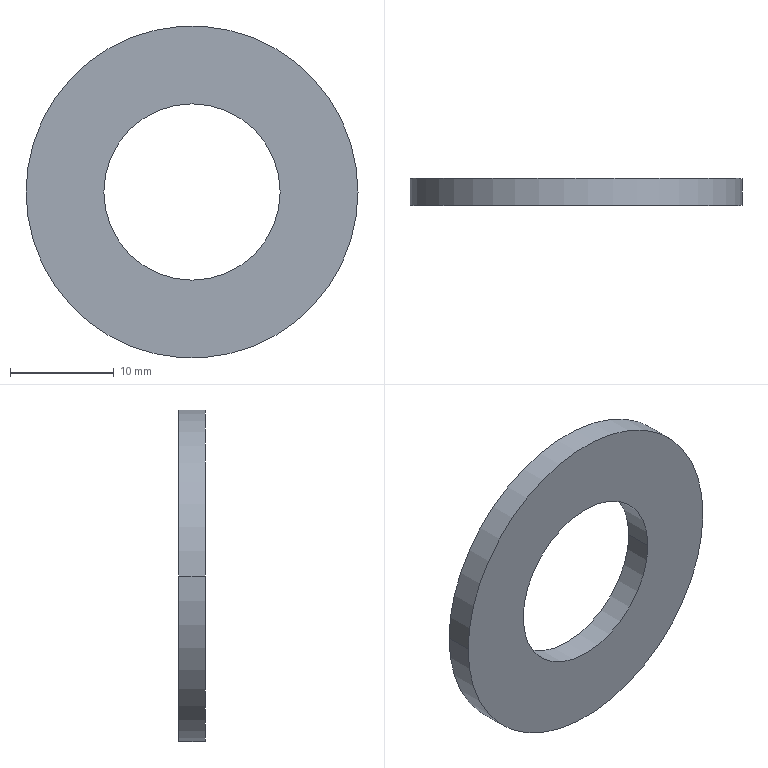Part | STEP file | ZZ21-M16 | 1 solid | 6 faces | box 32 x 2.6 x 32 mm | volume 1501 mm3 | cylinder 4 | plane 2 | commonest cylinder face diameters 17 x2 32 x2
STEP:
#1=CARTESIAN_POINT('',(0.,0.,0.));
#2=DIRECTION('',(0.,0.,1.));
#3=DIRECTION('',(1.,0.,0.));
#4=AXIS2_PLACEMENT_3D('',#1,#2,#3);
#5=CARTESIAN_POINT('',(-8.5,0.,0.));
#6=VERTEX_POINT('',#5);
#7=CARTESIAN_POINT('',(-8.5,2.6,0.));
#8=VERTEX_POINT('',#7);
#9=CARTESIAN_POINT('',(-8.5,0.,0.));
#10=DIRECTION('',(0.,1.,0.));
#11=VECTOR('',#10,1.);
#12=LINE('',#9,#11);
#13=CARTESIAN_POINT('',(0.,0.,0.));
#14=DIRECTION('',(0.,1.,0.));
#15=DIRECTION('',(-1.,0.,0.));
#16=AXIS2_PLACEMENT_3D('',#13,#14,#15);
#17=CYLINDRICAL_SURFACE('',#16,8.5);
#18=CARTESIAN_POINT('',(6.283,0.));
#19=DIRECTION('',(0.,1.));
#20=VECTOR('',#19,1.);
#21=LINE('',#18,#20);
#22=(GEOMETRIC_REPRESENTATION_CONTEXT(2)PARAMETRIC_REPRESENTATION_CONTEXT()REPRESENTATION_CONTEXT('',''));
#23=DEFINITIONAL_REPRESENTATION('',(#21),#22);
#24=PCURVE('',#17,#23);
#25=CARTESIAN_POINT('',(0.,0.,0.));
#26=DIRECTION('',(0.,1.,0.));
#27=DIRECTION('',(-1.,0.,0.));
#28=AXIS2_PLACEMENT_3D('',#25,#26,#27);
#29=CYLINDRICAL_SURFACE('',#28,8.5);
#30=CARTESIAN_POINT('',(0.,0.));
#31=DIRECTION('',(0.,1.));
#32=VECTOR('',#31,1.);
#33=LINE('',#30,#32);
#34=(GEOMETRIC_REPRESENTATION_CONTEXT(2)PARAMETRIC_REPRESENTATION_CONTEXT()REPRESENTATION_CONTEXT('',''));
#35=DEFINITIONAL_REPRESENTATION('',(#33),#34);
#36=PCURVE('',#29,#35);
#37=SURFACE_CURVE('',#12,(#24,#36),.PCURVE_S1.);
#38=EDGE_CURVE('',#6,#8,#37,.T.);
#39=ORIENTED_EDGE('',*,*,#38,.T.);
#40=CARTESIAN_POINT('',(8.5,2.6,0.));
#41=VERTEX_POINT('',#40);
#42=CARTESIAN_POINT('',(0.,2.6,0.));
#43=DIRECTION('',(0.,-1.,0.));
#44=DIRECTION('',(1.,0.,0.));
#45=AXIS2_PLACEMENT_3D('',#42,#43,#44);
#46=CIRCLE('',#45,8.5);
#47=CARTESIAN_POINT('',(9.425,2.6));
#48=DIRECTION('',(-1.,0.));
#49=VECTOR('',#48,1.);
#50=LINE('',#47,#49);
#51=(GEOMETRIC_REPRESENTATION_CONTEXT(2)PARAMETRIC_REPRESENTATION_CONTEXT()REPRESENTATION_CONTEXT('',''));
#52=DEFINITIONAL_REPRESENTATION('',(#50),#51);
#53=PCURVE('',#17,#52);
#54=CARTESIAN_POINT('',(0.,2.6,0.));
#55=DIRECTION('',(0.,1.,0.));
#56=DIRECTION('',(-1.,0.,0.));
#57=AXIS2_PLACEMENT_3D('',#54,#55,#56);
#58=PLANE('',#57);
#59=CARTESIAN_POINT('',(-8.5,0.));
#60=CARTESIAN_POINT('',(-8.5,14.722));
#61=CARTESIAN_POINT('',(4.25,7.361));
#62=CARTESIAN_POINT('',(17.,0.));
#63=CARTESIAN_POINT('',(4.25,-7.361));
#64=CARTESIAN_POINT('',(-8.5,-14.722));
#65=CARTESIAN_POINT('',(-8.5,0.));
#66=(BOUNDED_CURVE()B_SPLINE_CURVE(2,(#59,#60,#61,#62,#63,#64,#65),.UNSPECIFIED.,.T.,.F.)B_SPLINE_CURVE_WITH_KNOTS((1,2,2,2,2,1),(-2.094,0.,2.094,4.189,6.283,8.378),.UNSPECIFIED.)CURVE()GEOMETRIC_REPRESENTATION_ITEM()RATIONAL_B_SPLINE_CURVE((1.,0.5,1.,0.5,1.,0.5,1.))REPRESENTATION_ITEM(''));
#67=(GEOMETRIC_REPRESENTATION_CONTEXT(2)PARAMETRIC_REPRESENTATION_CONTEXT()REPRESENTATION_CONTEXT('',''));
#68=DEFINITIONAL_REPRESENTATION('',(#66),#67);
#69=PCURVE('',#58,#68);
#70=SURFACE_CURVE('',#46,(#53,#69),.PCURVE_S1.);
#71=EDGE_CURVE('',#8,#41,#70,.T.);
#72=ORIENTED_EDGE('',*,*,#71,.T.);
#73=CARTESIAN_POINT('',(8.5,0.,0.));
#74=VERTEX_POINT('',#73);
#75=CARTESIAN_POINT('',(8.5,0.,0.));
#76=DIRECTION('',(0.,1.,0.));
#77=VECTOR('',#76,1.);
#78=LINE('',#75,#77);
#79=CARTESIAN_POINT('',(3.142,0.));
#80=DIRECTION('',(0.,1.));
#81=VECTOR('',#80,1.);
#82=LINE('',#79,#81);
#83=(GEOMETRIC_REPRESENTATION_CONTEXT(2)PARAMETRIC_REPRESENTATION_CONTEXT()REPRESENTATION_CONTEXT('',''));
#84=DEFINITIONAL_REPRESENTATION('',(#82),#83);
#85=PCURVE('',#17,#84);
#86=CARTESIAN_POINT('',(3.142,0.));
#87=DIRECTION('',(0.,1.));
#88=VECTOR('',#87,1.);
#89=LINE('',#86,#88);
#90=(GEOMETRIC_REPRESENTATION_CONTEXT(2)PARAMETRIC_REPRESENTATION_CONTEXT()REPRESENTATION_CONTEXT('',''));
#91=DEFINITIONAL_REPRESENTATION('',(#89),#90);
#92=PCURVE('',#29,#91);
#93=SURFACE_CURVE('',#78,(#85,#92),.PCURVE_S1.);
#94=EDGE_CURVE('',#74,#41,#93,.T.);
#95=ORIENTED_EDGE('',*,*,#94,.F.);
#96=CARTESIAN_POINT('',(0.,0.,0.));
#97=DIRECTION('',(0.,1.,0.));
#98=DIRECTION('',(-1.,0.,0.));
#99=AXIS2_PLACEMENT_3D('',#96,#97,#98);
#100=CIRCLE('',#99,8.5);
#101=CARTESIAN_POINT('',(0.,0.));
#102=DIRECTION('',(1.,0.));
#103=VECTOR('',#102,1.);
#104=LINE('',#101,#103);
#105=(GEOMETRIC_REPRESENTATION_CONTEXT(2)PARAMETRIC_REPRESENTATION_CONTEXT()REPRESENTATION_CONTEXT('',''));
#106=DEFINITIONAL_REPRESENTATION('',(#104),#105);
#107=PCURVE('',#17,#106);
#108=CARTESIAN_POINT('',(0.,0.,0.));
#109=DIRECTION('',(0.,-1.,0.));
#110=DIRECTION('',(1.,0.,0.));
#111=AXIS2_PLACEMENT_3D('',#108,#109,#110);
#112=PLANE('',#111);
#113=CARTESIAN_POINT('',(-8.5,0.));
#114=CARTESIAN_POINT('',(-8.5,14.722));
#115=CARTESIAN_POINT('',(4.25,7.361));
#116=CARTESIAN_POINT('',(17.,0.));
#117=CARTESIAN_POINT('',(4.25,-7.361));
#118=CARTESIAN_POINT('',(-8.5,-14.722));
#119=CARTESIAN_POINT('',(-8.5,0.));
#120=(BOUNDED_CURVE()B_SPLINE_CURVE(2,(#113,#114,#115,#116,#117,#118,#119),.UNSPECIFIED.,.T.,.F.)B_SPLINE_CURVE_WITH_KNOTS((1,2,2,2,2,1),(-2.094,0.,2.094,4.189,6.283,8.378),.UNSPECIFIED.)CURVE()GEOMETRIC_REPRESENTATION_ITEM()RATIONAL_B_SPLINE_CURVE((1.,0.5,1.,0.5,1.,0.5,1.))REPRESENTATION_ITEM(''));
#121=(GEOMETRIC_REPRESENTATION_CONTEXT(2)PARAMETRIC_REPRESENTATION_CONTEXT()REPRESENTATION_CONTEXT('',''));
#122=DEFINITIONAL_REPRESENTATION('',(#120),#121);
#123=PCURVE('',#112,#122);
#124=SURFACE_CURVE('',#100,(#107,#123),.PCURVE_S1.);
#125=EDGE_CURVE('',#74,#6,#124,.T.);
#126=ORIENTED_EDGE('',*,*,#125,.T.);
#127=EDGE_LOOP('',(#39,#72,#95,#126));
#128=FACE_BOUND('',#127,.F.);
#129=ADVANCED_FACE('',(#128),#17,.F.);
#130=CARTESIAN_POINT('',(-16.,0.,0.));
#131=VERTEX_POINT('',#130);
#132=CARTESIAN_POINT('',(16.,0.,0.));
#133=VERTEX_POINT('',#132);
#134=CARTESIAN_POINT('',(0.,0.,0.));
#135=DIRECTION('',(0.,1.,0.));
#136=DIRECTION('',(-1.,0.,0.));
#137=AXIS2_PLACEMENT_3D('',#134,#135,#136);
#138=CIRCLE('',#137,16.);
#139=CARTESIAN_POINT('',(0.,0.,0.));
#140=DIRECTION('',(0.,1.,0.));
#141=DIRECTION('',(-1.,0.,0.));
#142=AXIS2_PLACEMENT_3D('',#139,#140,#141);
#143=CYLINDRICAL_SURFACE('',#142,16.);
#144=CARTESIAN_POINT('',(0.,0.));
#145=DIRECTION('',(1.,0.));
#146=VECTOR('',#145,1.);
#147=LINE('',#144,#146);
#148=(GEOMETRIC_REPRESENTATION_CONTEXT(2)PARAMETRIC_REPRESENTATION_CONTEXT()REPRESENTATION_CONTEXT('',''));
#149=DEFINITIONAL_REPRESENTATION('',(#147),#148);
#150=PCURVE('',#143,#149);
#151=CARTESIAN_POINT('',(-16.,0.));
#152=CARTESIAN_POINT('',(-16.,27.713));
#153=CARTESIAN_POINT('',(8.,13.856));
#154=CARTESIAN_POINT('',(32.,0.));
#155=CARTESIAN_POINT('',(8.,-13.856));
#156=CARTESIAN_POINT('',(-16.,-27.713));
#157=CARTESIAN_POINT('',(-16.,0.));
#158=(BOUNDED_CURVE()B_SPLINE_CURVE(2,(#151,#152,#153,#154,#155,#156,#157),.UNSPECIFIED.,.T.,.F.)B_SPLINE_CURVE_WITH_KNOTS((1,2,2,2,2,1),(-2.094,0.,2.094,4.189,6.283,8.378),.UNSPECIFIED.)CURVE()GEOMETRIC_REPRESENTATION_ITEM()RATIONAL_B_SPLINE_CURVE((1.,0.5,1.,0.5,1.,0.5,1.))REPRESENTATION_ITEM(''));
#159=(GEOMETRIC_REPRESENTATION_CONTEXT(2)PARAMETRIC_REPRESENTATION_CONTEXT()REPRESENTATION_CONTEXT('',''));
#160=DEFINITIONAL_REPRESENTATION('',(#158),#159);
#161=PCURVE('',#112,#160);
#162=SURFACE_CURVE('',#138,(#150,#161),.PCURVE_S1.);
#163=EDGE_CURVE('',#131,#133,#162,.T.);
#164=ORIENTED_EDGE('',*,*,#163,.T.);
#165=CARTESIAN_POINT('',(16.,2.6,0.));
#166=VERTEX_POINT('',#165);
#167=CARTESIAN_POINT('',(16.,0.,0.));
#168=DIRECTION('',(0.,1.,0.));
#169=VECTOR('',#168,1.);
#170=LINE('',#167,#169);
#171=CARTESIAN_POINT('',(3.142,0.));
#172=DIRECTION('',(0.,1.));
#173=VECTOR('',#172,1.);
#174=LINE('',#171,#173);
#175=(GEOMETRIC_REPRESENTATION_CONTEXT(2)PARAMETRIC_REPRESENTATION_CONTEXT()REPRESENTATION_CONTEXT('',''));
#176=DEFINITIONAL_REPRESENTATION('',(#174),#175);
#177=PCURVE('',#143,#176);
#178=CARTESIAN_POINT('',(0.,0.,0.));
#179=DIRECTION('',(0.,1.,0.));
#180=DIRECTION('',(-1.,0.,0.));
#181=AXIS2_PLACEMENT_3D('',#178,#179,#180);
#182=CYLINDRICAL_SURFACE('',#181,16.);
#183=CARTESIAN_POINT('',(3.142,0.));
#184=DIRECTION('',(0.,1.));
#185=VECTOR('',#184,1.);
#186=LINE('',#183,#185);
#187=(GEOMETRIC_REPRESENTATION_CONTEXT(2)PARAMETRIC_REPRESENTATION_CONTEXT()REPRESENTATION_CONTEXT('',''));
#188=DEFINITIONAL_REPRESENTATION('',(#186),#187);
#189=PCURVE('',#182,#188);
#190=SURFACE_CURVE('',#170,(#177,#189),.PCURVE_S1.);
#191=EDGE_CURVE('',#133,#166,#190,.T.);
#192=ORIENTED_EDGE('',*,*,#191,.T.);
#193=CARTESIAN_POINT('',(-16.,2.6,0.));
#194=VERTEX_POINT('',#193);
#195=CARTESIAN_POINT('',(0.,2.6,0.));
#196=DIRECTION('',(0.,-1.,0.));
#197=DIRECTION('',(1.,0.,0.));
#198=AXIS2_PLACEMENT_3D('',#195,#196,#197);
#199=CIRCLE('',#198,16.);
#200=CARTESIAN_POINT('',(3.142,2.6));
#201=DIRECTION('',(-1.,0.));
#202=VECTOR('',#201,1.);
#203=LINE('',#200,#202);
#204=(GEOMETRIC_REPRESENTATION_CONTEXT(2)PARAMETRIC_REPRESENTATION_CONTEXT()REPRESENTATION_CONTEXT('',''));
#205=DEFINITIONAL_REPRESENTATION('',(#203),#204);
#206=PCURVE('',#143,#205);
#207=CARTESIAN_POINT('',(-16.,0.));
#208=CARTESIAN_POINT('',(-16.,27.713));
#209=CARTESIAN_POINT('',(8.,13.856));
#210=CARTESIAN_POINT('',(32.,0.));
#211=CARTESIAN_POINT('',(8.,-13.856));
#212=CARTESIAN_POINT('',(-16.,-27.713));
#213=CARTESIAN_POINT('',(-16.,0.));
#214=(BOUNDED_CURVE()B_SPLINE_CURVE(2,(#207,#208,#209,#210,#211,#212,#213),.UNSPECIFIED.,.T.,.F.)B_SPLINE_CURVE_WITH_KNOTS((1,2,2,2,2,1),(-2.094,0.,2.094,4.189,6.283,8.378),.UNSPECIFIED.)CURVE()GEOMETRIC_REPRESENTATION_ITEM()RATIONAL_B_SPLINE_CURVE((1.,0.5,1.,0.5,1.,0.5,1.))REPRESENTATION_ITEM(''));
#215=(GEOMETRIC_REPRESENTATION_CONTEXT(2)PARAMETRIC_REPRESENTATION_CONTEXT()REPRESENTATION_CONTEXT('',''));
#216=DEFINITIONAL_REPRESENTATION('',(#214),#215);
#217=PCURVE('',#58,#216);
#218=SURFACE_CURVE('',#199,(#206,#217),.PCURVE_S1.);
#219=EDGE_CURVE('',#166,#194,#218,.T.);
#220=ORIENTED_EDGE('',*,*,#219,.T.);
#221=CARTESIAN_POINT('',(-16.,0.,0.));
#222=DIRECTION('',(0.,1.,0.));
#223=VECTOR('',#222,1.);
#224=LINE('',#221,#223);
#225=CARTESIAN_POINT('',(0.,0.));
#226=DIRECTION('',(0.,1.));
#227=VECTOR('',#226,1.);
#228=LINE('',#225,#227);
#229=(GEOMETRIC_REPRESENTATION_CONTEXT(2)PARAMETRIC_REPRESENTATION_CONTEXT()REPRESENTATION_CONTEXT('',''));
#230=DEFINITIONAL_REPRESENTATION('',(#228),#229);
#231=PCURVE('',#143,#230);
#232=CARTESIAN_POINT('',(6.283,0.));
#233=DIRECTION('',(0.,1.));
#234=VECTOR('',#233,1.);
#235=LINE('',#232,#234);
#236=(GEOMETRIC_REPRESENTATION_CONTEXT(2)PARAMETRIC_REPRESENTATION_CONTEXT()REPRESENTATION_CONTEXT('',''));
#237=DEFINITIONAL_REPRESENTATION('',(#235),#236);
#238=PCURVE('',#182,#237);
#239=SURFACE_CURVE('',#224,(#231,#238),.PCURVE_S1.);
#240=EDGE_CURVE('',#131,#194,#239,.T.);
#241=ORIENTED_EDGE('',*,*,#240,.F.);
#242=EDGE_LOOP('',(#164,#192,#220,#241));
#243=FACE_BOUND('',#242,.T.);
#244=ADVANCED_FACE('',(#243),#143,.T.);
#245=ORIENTED_EDGE('',*,*,#71,.T.);
#246=CARTESIAN_POINT('',(0.,2.6,0.));
#247=DIRECTION('',(0.,-1.,0.));
#248=DIRECTION('',(1.,0.,0.));
#249=AXIS2_PLACEMENT_3D('',#246,#247,#248);
#250=CIRCLE('',#249,8.5);
#251=CARTESIAN_POINT('',(-8.5,0.));
#252=CARTESIAN_POINT('',(-8.5,14.722));
#253=CARTESIAN_POINT('',(4.25,7.361));
#254=CARTESIAN_POINT('',(17.,0.));
#255=CARTESIAN_POINT('',(4.25,-7.361));
#256=CARTESIAN_POINT('',(-8.5,-14.722));
#257=CARTESIAN_POINT('',(-8.5,0.));
#258=(BOUNDED_CURVE()B_SPLINE_CURVE(2,(#251,#252,#253,#254,#255,#256,#257),.UNSPECIFIED.,.T.,.F.)B_SPLINE_CURVE_WITH_KNOTS((1,2,2,2,2,1),(-2.094,0.,2.094,4.189,6.283,8.378),.UNSPECIFIED.)CURVE()GEOMETRIC_REPRESENTATION_ITEM()RATIONAL_B_SPLINE_CURVE((1.,0.5,1.,0.5,1.,0.5,1.))REPRESENTATION_ITEM(''));
#259=(GEOMETRIC_REPRESENTATION_CONTEXT(2)PARAMETRIC_REPRESENTATION_CONTEXT()REPRESENTATION_CONTEXT('',''));
#260=DEFINITIONAL_REPRESENTATION('',(#258),#259);
#261=PCURVE('',#58,#260);
#262=CARTESIAN_POINT('',(3.142,2.6));
#263=DIRECTION('',(-1.,0.));
#264=VECTOR('',#263,1.);
#265=LINE('',#262,#264);
#266=(GEOMETRIC_REPRESENTATION_CONTEXT(2)PARAMETRIC_REPRESENTATION_CONTEXT()REPRESENTATION_CONTEXT('',''));
#267=DEFINITIONAL_REPRESENTATION('',(#265),#266);
#268=PCURVE('',#29,#267);
#269=SURFACE_CURVE('',#250,(#261,#268),.PCURVE_S1.);
#270=EDGE_CURVE('',#41,#8,#269,.T.);
#271=ORIENTED_EDGE('',*,*,#270,.T.);
#272=EDGE_LOOP('',(#245,#271));
#273=FACE_BOUND('',#272,.T.);
#274=CARTESIAN_POINT('',(0.,2.6,0.));
#275=DIRECTION('',(0.,-1.,0.));
#276=DIRECTION('',(1.,0.,0.));
#277=AXIS2_PLACEMENT_3D('',#274,#275,#276);
#278=CIRCLE('',#277,16.);
#279=CARTESIAN_POINT('',(-16.,0.));
#280=CARTESIAN_POINT('',(-16.,27.713));
#281=CARTESIAN_POINT('',(8.,13.856));
#282=CARTESIAN_POINT('',(32.,0.));
#283=CARTESIAN_POINT('',(8.,-13.856));
#284=CARTESIAN_POINT('',(-16.,-27.713));
#285=CARTESIAN_POINT('',(-16.,0.));
#286=(BOUNDED_CURVE()B_SPLINE_CURVE(2,(#279,#280,#281,#282,#283,#284,#285),.UNSPECIFIED.,.T.,.F.)B_SPLINE_CURVE_WITH_KNOTS((1,2,2,2,2,1),(-2.094,0.,2.094,4.189,6.283,8.378),.UNSPECIFIED.)CURVE()GEOMETRIC_REPRESENTATION_ITEM()RATIONAL_B_SPLINE_CURVE((1.,0.5,1.,0.5,1.,0.5,1.))REPRESENTATION_ITEM(''));
#287=(GEOMETRIC_REPRESENTATION_CONTEXT(2)PARAMETRIC_REPRESENTATION_CONTEXT()REPRESENTATION_CONTEXT('',''));
#288=DEFINITIONAL_REPRESENTATION('',(#286),#287);
#289=PCURVE('',#58,#288);
#290=CARTESIAN_POINT('',(9.425,2.6));
#291=DIRECTION('',(-1.,0.));
#292=VECTOR('',#291,1.);
#293=LINE('',#290,#292);
#294=(GEOMETRIC_REPRESENTATION_CONTEXT(2)PARAMETRIC_REPRESENTATION_CONTEXT()REPRESENTATION_CONTEXT('',''));
#295=DEFINITIONAL_REPRESENTATION('',(#293),#294);
#296=PCURVE('',#182,#295);
#297=SURFACE_CURVE('',#278,(#289,#296),.PCURVE_S1.);
#298=EDGE_CURVE('',#194,#166,#297,.T.);
#299=ORIENTED_EDGE('',*,*,#298,.F.);
#300=ORIENTED_EDGE('',*,*,#219,.F.);
#301=EDGE_LOOP('',(#299,#300));
#302=FACE_BOUND('',#301,.T.);
#303=ADVANCED_FACE('',(#273,#302),#58,.T.);
#304=CARTESIAN_POINT('',(0.,0.,0.));
#305=DIRECTION('',(0.,1.,0.));
#306=DIRECTION('',(-1.,0.,0.));
#307=AXIS2_PLACEMENT_3D('',#304,#305,#306);
#308=CIRCLE('',#307,8.5);
#309=CARTESIAN_POINT('',(-8.5,0.));
#310=CARTESIAN_POINT('',(-8.5,14.722));
#311=CARTESIAN_POINT('',(4.25,7.361));
#312=CARTESIAN_POINT('',(17.,0.));
#313=CARTESIAN_POINT('',(4.25,-7.361));
#314=CARTESIAN_POINT('',(-8.5,-14.722));
#315=CARTESIAN_POINT('',(-8.5,0.));
#316=(BOUNDED_CURVE()B_SPLINE_CURVE(2,(#309,#310,#311,#312,#313,#314,#315),.UNSPECIFIED.,.T.,.F.)B_SPLINE_CURVE_WITH_KNOTS((1,2,2,2,2,1),(-2.094,0.,2.094,4.189,6.283,8.378),.UNSPECIFIED.)CURVE()GEOMETRIC_REPRESENTATION_ITEM()RATIONAL_B_SPLINE_CURVE((1.,0.5,1.,0.5,1.,0.5,1.))REPRESENTATION_ITEM(''));
#317=(GEOMETRIC_REPRESENTATION_CONTEXT(2)PARAMETRIC_REPRESENTATION_CONTEXT()REPRESENTATION_CONTEXT('',''));
#318=DEFINITIONAL_REPRESENTATION('',(#316),#317);
#319=PCURVE('',#112,#318);
#320=CARTESIAN_POINT('',(0.,0.));
#321=DIRECTION('',(1.,0.));
#322=VECTOR('',#321,1.);
#323=LINE('',#320,#322);
#324=(GEOMETRIC_REPRESENTATION_CONTEXT(2)PARAMETRIC_REPRESENTATION_CONTEXT()REPRESENTATION_CONTEXT('',''));
#325=DEFINITIONAL_REPRESENTATION('',(#323),#324);
#326=PCURVE('',#29,#325);
#327=SURFACE_CURVE('',#308,(#319,#326),.PCURVE_S1.);
#328=EDGE_CURVE('',#6,#74,#327,.T.);
#329=ORIENTED_EDGE('',*,*,#328,.T.);
#330=ORIENTED_EDGE('',*,*,#125,.T.);
#331=EDGE_LOOP('',(#329,#330));
#332=FACE_BOUND('',#331,.T.);
#333=ORIENTED_EDGE('',*,*,#163,.F.);
#334=CARTESIAN_POINT('',(0.,0.,0.));
#335=DIRECTION('',(0.,1.,0.));
#336=DIRECTION('',(-1.,0.,0.));
#337=AXIS2_PLACEMENT_3D('',#334,#335,#336);
#338=CIRCLE('',#337,16.);
#339=CARTESIAN_POINT('',(-16.,0.));
#340=CARTESIAN_POINT('',(-16.,27.713));
#341=CARTESIAN_POINT('',(8.,13.856));
#342=CARTESIAN_POINT('',(32.,0.));
#343=CARTESIAN_POINT('',(8.,-13.856));
#344=CARTESIAN_POINT('',(-16.,-27.713));
#345=CARTESIAN_POINT('',(-16.,0.));
#346=(BOUNDED_CURVE()B_SPLINE_CURVE(2,(#339,#340,#341,#342,#343,#344,#345),.UNSPECIFIED.,.T.,.F.)B_SPLINE_CURVE_WITH_KNOTS((1,2,2,2,2,1),(-2.094,0.,2.094,4.189,6.283,8.378),.UNSPECIFIED.)CURVE()GEOMETRIC_REPRESENTATION_ITEM()RATIONAL_B_SPLINE_CURVE((1.,0.5,1.,0.5,1.,0.5,1.))REPRESENTATION_ITEM(''));
#347=(GEOMETRIC_REPRESENTATION_CONTEXT(2)PARAMETRIC_REPRESENTATION_CONTEXT()REPRESENTATION_CONTEXT('',''));
#348=DEFINITIONAL_REPRESENTATION('',(#346),#347);
#349=PCURVE('',#112,#348);
#350=CARTESIAN_POINT('',(0.,0.));
#351=DIRECTION('',(1.,0.));
#352=VECTOR('',#351,1.);
#353=LINE('',#350,#352);
#354=(GEOMETRIC_REPRESENTATION_CONTEXT(2)PARAMETRIC_REPRESENTATION_CONTEXT()REPRESENTATION_CONTEXT('',''));
#355=DEFINITIONAL_REPRESENTATION('',(#353),#354);
#356=PCURVE('',#182,#355);
#357=SURFACE_CURVE('',#338,(#349,#356),.PCURVE_S1.);
#358=EDGE_CURVE('',#133,#131,#357,.T.);
#359=ORIENTED_EDGE('',*,*,#358,.F.);
#360=EDGE_LOOP('',(#333,#359));
#361=FACE_BOUND('',#360,.T.);
#362=ADVANCED_FACE('',(#332,#361),#112,.T.);
#363=ORIENTED_EDGE('',*,*,#191,.F.);
#364=ORIENTED_EDGE('',*,*,#358,.T.);
#365=ORIENTED_EDGE('',*,*,#240,.T.);
#366=ORIENTED_EDGE('',*,*,#298,.T.);
#367=EDGE_LOOP('',(#363,#364,#365,#366));
#368=FACE_BOUND('',#367,.T.);
#369=ADVANCED_FACE('',(#368),#182,.T.);
#370=ORIENTED_EDGE('',*,*,#270,.T.);
#371=ORIENTED_EDGE('',*,*,#38,.F.);
#372=ORIENTED_EDGE('',*,*,#328,.T.);
#373=ORIENTED_EDGE('',*,*,#94,.T.);
#374=EDGE_LOOP('',(#370,#371,#372,#373));
#375=FACE_BOUND('',#374,.F.);
#376=ADVANCED_FACE('',(#375),#29,.F.);
#377=CLOSED_SHELL('',(#129,#244,#303,#362,#369,#376));
#378=MANIFOLD_SOLID_BREP('',#377);
#379=(LENGTH_UNIT()NAMED_UNIT(*)SI_UNIT(.MILLI.,.METRE.));
#380=UNCERTAINTY_MEASURE_WITH_UNIT(LENGTH_MEASURE(0.0000001),#379,'','');
#381=(NAMED_UNIT(*)PLANE_ANGLE_UNIT()SI_UNIT($,.RADIAN.));
#382=(NAMED_UNIT(*)SI_UNIT($,.STERADIAN.)SOLID_ANGLE_UNIT());
#383=(GEOMETRIC_REPRESENTATION_CONTEXT(3)GLOBAL_UNCERTAINTY_ASSIGNED_CONTEXT((#380))GLOBAL_UNIT_ASSIGNED_CONTEXT((#379,#381,#382))REPRESENTATION_CONTEXT('',''));
#384=ADVANCED_BREP_SHAPE_REPRESENTATION('',(#4,#378),#383);